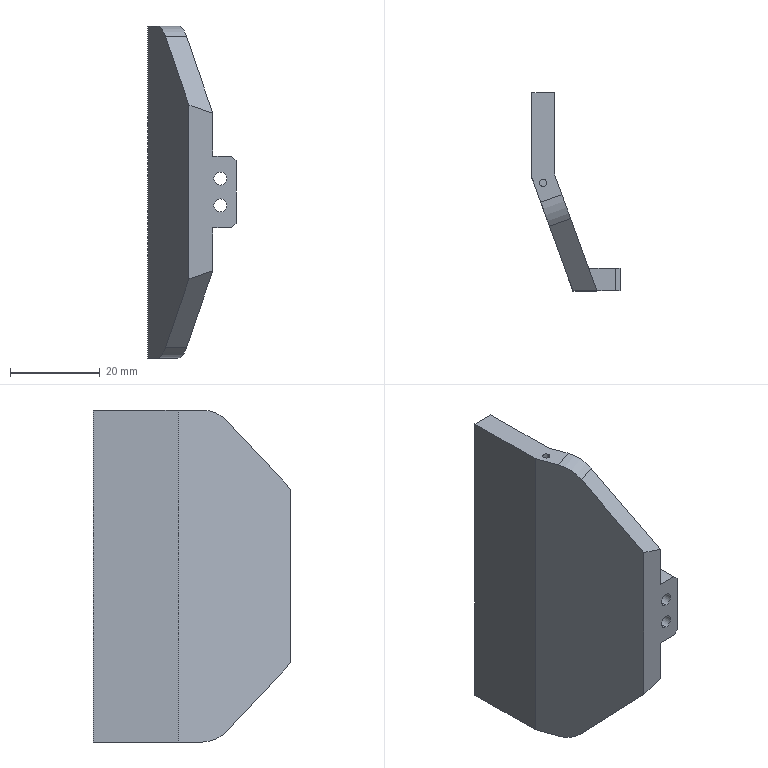NC program | NX | posted with a generic post | part box 19.643 x 44.061 x 74 mm
Lines 6014 to 6515 of 6515:
(FLOOR_FACING , TOOL : D8精光)
N12026 T03 M6
N12028 G54
N12030 G17 G0 G90 X-46. Y40.058 B0. C0. S5500 M3
N12032 G43 Z30. H3
N12034 Z-12.643
N12036 G94 G1 Z-14.643 F800.
N12038 X-41.
N12040 X41.
N12042 Y35.029
N12044 X-41.
N12046 Y30.
N12048 X41.
N12050 X43.
N12052 Z-12.643
N12054 G0 Z30.
(FLOOR_FACING_COPY , TOOL : D8精光)
N12056 X13. Y2.
N12058 Z2.
N12060 G1 Z0.
N12062 X11.
N12064 X-11.
N12066 X-13.
N12068 Z2.
N12070 G0 Z30.
(PLANAR_MILL_6_COPY , TOOL : D8精光)
N12072 X-12. Y9. S4500
N12074 Z-5.
N12076 G1 Z-7.
N12078 X-8.
N12080 X8.
N12082 X12.
N12084 Z-5.
N12086 G0 Z30.
N12088 X-12.
N12090 Z-5.
N12092 G1 Z-7.
N12094 X-8.
N12096 X8.
N12098 X12.
N12100 Z-5.
N12102 G0 Z30.
(PLANAR_MILL_6 , TOOL : D8精光)
N12104 X43. Y40.118
N12106 Z-19.
N12108 G1 Z-21.
N12110 G3 X41. Y38.118 R2.
N12112 G1 Y19.674
N12114 G2 X40.986 Y19.34 R4.
N12116 X37.617 Y11.668 R10.966
N12118 X37.396 Y11.444 R4.
N12120 G1 X22.116 Y-2.915
N12122 G2 X19.377 Y-4. R4.
N12124 G1 X-19.377
N12126 G2 X-22.116 Y-2.915 R4.
N12128 G1 X-37.396 Y11.444
N12130 G2 X-37.617 Y11.668 R4.
N12132 X-40.986 Y19.34 R11.02
N12134 X-41. Y19.674 R4.
N12136 G1 Y38.118
N12138 G3 X-43. Y40.118 R2.
N12140 G1 Z-19.
N12142 G0 Z30.
N12144 X43.
N12146 Z-19.
N12148 G1 Z-21.
N12150 G3 X41. Y38.118 R2.
N12152 G1 Y19.674
N12154 G2 X40.986 Y19.34 R4.
N12156 X37.617 Y11.668 R10.966
N12158 X37.396 Y11.444 R4.
N12160 G1 X22.116 Y-2.915
N12162 G2 X19.377 Y-4. R4.
N12164 G1 X-19.377
N12166 G2 X-22.116 Y-2.915 R4.
N12168 G1 X-37.396 Y11.444
N12170 G2 X-37.617 Y11.668 R4.
N12172 X-40.986 Y19.34 R11.02
N12174 X-41. Y19.674 R4.
N12176 G1 Y38.118
N12178 G3 X-43. Y40.118 R2.
N12180 G1 Z-19.
N12182 G0 Z30.
N12184 M5
(CURVE_DRIVE_1 , TOOL : R1)
N12186 T04 M6
N12188 G54
N12190 G17 G0 G90 X-7.728 Y6.011 B0. C0. S4500 M3
N12192 G43 Z30. H4
N12194 Z2.798
N12196 G94 G1 Z0.675 F1000.
N12198 Y5.999 Z0.532
N12200 Y5.967 Z0.393
N12202 Y5.916 Z0.26
N12204 Y5.846 Z0.136
N12206 Y5.759 Z0.022
N12208 Y5.657 Z-0.077
N12210 Y5.542 Z-0.162
N12212 Y5.416 Z-0.229
N12214 Y5.282 Z-0.277
N12216 Y5.142 Z-0.306
N12218 Y5. Z-0.315
N12220 Y4.958 Z-0.314
N12222 Y0.043
N12224 Y0. Z-0.315
N12226 X-7.749 Z-0.336
N12228 Y0.041 Z-0.335
N12230 Y4.958
N12232 Y5. Z-0.336
N12234 X-7.771 Z-0.357
N12236 Y4.958 Z-0.356
N12238 Y0.043
N12240 Y0. Z-0.357
N12242 X-7.792 Z-0.378
N12244 Y0.043
N12246 Y4.958
N12248 Y5.
N12250 X-7.813 Z-0.399
N12252 Y4.958
N12254 Y0.043
N12256 Y0.
N12258 X-7.834 Z-0.42
N12260 Y0.043
N12262 Y4.958
N12264 Y5.
N12266 X-7.855 Z-0.442
N12268 Y4.958 Z-0.441
N12270 Y0.043
N12272 Y0. Z-0.442
N12274 X-7.877 Z-0.463
N12276 Y0.043 Z-0.462
N12278 Y4.958
N12280 Y5. Z-0.463
N12282 X-7.898 Z-0.484
N12284 Y4.955
N12286 Y0.041
N12288 Y0.
N12290 X-7.919 Z-0.505
N12292 Y0.043
N12294 Y4.958
N12296 Y5.
N12298 X-7.94 Z-0.526
N12300 Y4.958
N12302 Y0.043
N12304 Y0.
N12306 X-7.961 Z-0.548
N12308 Y0.043 Z-0.547
N12310 Y4.958
N12312 Y5. Z-0.548
N12314 X-7.983 Z-0.569
N12316 Y4.958 Z-0.568
N12318 Y0.043
N12320 Y0. Z-0.569
N12322 X-8.004 Z-0.59
N12324 Y0.043
N12326 Y4.958
N12328 Y5.
N12330 X-8.025 Z-0.611
N12332 Y4.958
N12334 Y0.043
N12336 Y0.
N12338 X-8.046 Z-0.633
N12340 Y0.043 Z-0.632
N12342 Y4.958
N12344 Y5. Z-0.633
N12346 X-8.068 Z-0.654
N12348 Y4.958 Z-0.653
N12350 Y0.043
N12352 Y0. Z-0.654
N12354 X-8.089 Z-0.675
N12356 Y0.043
N12358 Y4.958
N12360 Y5.
N12362 X-8.11 Z-0.696
N12364 Y4.958
N12366 Y0.043
N12368 Y0.
N12370 X-8.131 Z-0.717
N12372 Y0.043
N12374 Y4.958
N12376 Y5.
N12378 X-8.152 Z-0.739
N12380 Y4.958 Z-0.738
N12382 Y0.043
N12384 Y0. Z-0.739
N12386 X-8.174 Z-0.76
N12388 Y0.043 Z-0.759
N12390 Y4.958
N12392 Y5. Z-0.76
N12394 X-8.195 Z-0.781
N12396 Y4.958
N12398 Y0.043
N12400 Y0.
N12402 X-8.216 Z-0.802
N12404 Y0.043
N12406 Y4.958
N12408 Y5.
N12410 X-8.237 Z-0.823
N12412 Y4.958
N12414 Y0.043
N12416 Y0.
N12418 X-8.258 Z-0.845
N12420 Y0.043 Z-0.844
N12422 Y4.958
N12424 Y5. Z-0.845
N12426 X-8.28 Z-0.866
N12428 Y4.958 Z-0.865
N12430 Y0.043
N12432 Y0. Z-0.866
N12434 X-8.301 Z-0.887
N12436 Y0.043
N12438 Y4.958
N12440 Y5.
N12442 X-8.322 Z-0.908
N12444 Y4.958
N12446 Y0.043
N12448 Y0.
N12450 X-8.343 Z-0.93
N12452 Y0.043 Z-0.929
N12454 Y4.958
N12456 Y5. Z-0.93
N12458 X-8.364 Z-0.951
N12460 Y4.958 Z-0.95
N12462 X-8.365 Y0.043
N12464 Y0. Z-0.951
N12466 X-8.386 Z-0.972
N12468 Y0.043 Z-0.971
N12470 Y4.958
N12472 Y5. Z-0.972
N12474 X-8.407 Z-0.993
N12476 Y4.958
N12478 Y0.043
N12480 Y0.
N12482 X-8.428 Z-1.014
N12484 Y0.043
N12486 Y4.958
N12488 Y5.
N12490 X-8.449 Z-1.036
N12492 Y4.958 Z-1.035
N12494 Y0.043
N12496 Y0. Z-1.036
N12498 X-8.471 Z-1.057
N12500 Y0.043 Z-1.056
N12502 Y4.958
N12504 Y5. Z-1.057
N12506 X-8.492 Z-1.078
N12508 Y4.958
N12510 Y0.043
N12512 Y0.
N12514 X-8.513 Z-1.099
N12516 Y0.042
N12518 Y4.957
N12520 Y5.
N12522 X-8.534 Z-1.12
N12524 Y4.958
N12526 Y0.022
N12528 Y0.
N12530 X-8.555 Z-1.142
N12532 Y4.978 Z-1.141
N12534 Y5. Z-1.142
N12536 X-8.577 Z-1.163
N12538 Y4.958 Z-1.162
N12540 Y0. Z-1.163
N12542 X-8.598 Z-1.184
N12544 Y4.992
N12546 Y5.
N12548 X-8.619 Z-1.205
N12550 Y0.
N12552 X-8.64 Z-1.226
N12554 Y5.
N12556 X-8.661 Z-1.247
N12558 Y0.
N12560 X-8.682 Z-1.269
N12562 Y5.
N12564 X-8.703 Z-1.29
N12566 Y0.
N12568 Y-0.142 Z-1.282
N12570 Y-0.282 Z-1.253
N12572 Y-0.416 Z-1.204
N12574 Y-0.542 Z-1.137
N12576 Y-0.657 Z-1.053
N12578 Y-0.759 Z-0.953
N12580 Y-0.846 Z-0.84
N12582 Y-0.915 Z-0.715
N12584 Y-0.967 Z-0.582
N12586 Y-0.998 Z-0.443
N12588 Y-1.01 Z-0.301
N12590 Z2.472
N12592 G0 Z30.
N12594 X7.728 Y-1.011
N12596 Z2.798
N12598 G1 Z0.675
N12600 Y-0.999 Z0.532
N12602 Y-0.967 Z0.393
N12604 Y-0.916 Z0.26
N12606 Y-0.846 Z0.136
N12608 Y-0.759 Z0.022
N12610 Y-0.657 Z-0.077
N12612 Y-0.542 Z-0.162
N12614 Y-0.416 Z-0.229
N12616 Y-0.282 Z-0.277
N12618 Y-0.142 Z-0.306
N12620 Y0. Z-0.315
N12622 Y0.043 Z-0.314
N12624 Y4.958
N12626 Y5. Z-0.315
N12628 X7.749 Z-0.336
N12630 Y4.958 Z-0.335
N12632 Y0.043
N12634 Y0. Z-0.336
N12636 X7.771 Z-0.357
N12638 Y0.043 Z-0.356
N12640 Y4.958
N12642 Y5. Z-0.357
N12644 X7.792 Z-0.378
N12646 Y4.958
N12648 Y0.043
N12650 Y0.
N12652 X7.813 Z-0.399
N12654 Y0.043
N12656 Y4.958
N12658 Y5.
N12660 X7.834 Z-0.42
N12662 Y4.958
N12664 Y0.043
N12666 Y0.
N12668 X7.855 Z-0.442
N12670 Y0.043 Z-0.441
N12672 Y4.958
N12674 Y5. Z-0.442
N12676 X7.877 Z-0.463
N12678 Y4.958 Z-0.462
N12680 Y0.043
N12682 Y0. Z-0.463
N12684 X7.898 Z-0.484
N12686 Y0.045
N12688 Y4.959
N12690 Y5.
N12692 X7.919 Z-0.505
N12694 Y4.958
N12696 Y0.043
N12698 Y0.
N12700 X7.94 Z-0.526
N12702 Y0.043
N12704 Y4.958
N12706 Y5.
N12708 X7.961 Z-0.548
N12710 Y4.958 Z-0.547
N12712 Y0.043
N12714 Y0. Z-0.548
N12716 X7.983 Z-0.569
N12718 Y0.043 Z-0.568
N12720 Y4.958
N12722 Y5. Z-0.569
N12724 X8.004 Z-0.59
N12726 Y4.958
N12728 Y0.043
N12730 Y0.
N12732 X8.025 Z-0.611
N12734 Y0.043
N12736 Y4.958
N12738 Y5.
N12740 X8.046 Z-0.633
N12742 Y4.96 Z-0.632
N12744 Y0.043
N12746 Y0. Z-0.633
N12748 X8.068 Z-0.654
N12750 Y0.043 Z-0.653
N12752 Y4.958
N12754 Y5. Z-0.654
N12756 X8.089 Z-0.675
N12758 Y4.958
N12760 Y0.043
N12762 Y0.
N12764 X8.11 Z-0.696
N12766 Y0.043
N12768 Y4.958
N12770 Y5.
N12772 X8.131 Z-0.717
N12774 Y4.958
N12776 Y0.043
N12778 Y0.
N12780 X8.152 Z-0.739
N12782 Y0.043 Z-0.738
N12784 Y4.958
N12786 Y5. Z-0.739
N12788 X8.174 Z-0.76
N12790 Y4.958 Z-0.759
N12792 Y0.043
N12794 Y0. Z-0.76
N12796 X8.195 Z-0.781
N12798 Y0.043
N12800 Y4.958
N12802 Y5.
N12804 X8.216 Z-0.802
N12806 Y4.958
N12808 Y0.043
N12810 Y0.
N12812 X8.237 Z-0.823
N12814 Y0.043
N12816 Y4.958
N12818 Y5.
N12820 X8.258 Z-0.845
N12822 Y4.958 Z-0.844
N12824 Y0.043
N12826 Y0. Z-0.845
N12828 X8.28 Z-0.866
N12830 Y0.043 Z-0.865
N12832 Y4.958
N12834 Y5. Z-0.866
N12836 X8.301 Z-0.887
N12838 Y4.958
N12840 Y0.043
N12842 Y0.
N12844 X8.322 Z-0.908
N12846 Y0.043
N12848 Y4.958
N12850 Y5.
N12852 X8.343 Z-0.93
N12854 Y4.958 Z-0.929
N12856 Y0.043
N12858 Y0. Z-0.93
N12860 X8.365 Z-0.951
N12862 Y0.043 Z-0.95
N12864 Y4.96
N12866 Y5. Z-0.951
N12868 X8.386 Z-0.972
N12870 Y4.958
N12872 Y0.043
N12874 Y0.
N12876 X8.407 Z-0.993
N12878 Y0.043
N12880 Y4.958
N12882 Y5.
N12884 X8.428 Z-1.014
N12886 Y4.958
N12888 Y0.043
N12890 Y0.
N12892 X8.449 Z-1.036
N12894 Y0.043 Z-1.035
N12896 Y4.958
N12898 Y5. Z-1.036
N12900 X8.471 Z-1.057
N12902 Y4.958 Z-1.056
N12904 Y0.043
N12906 Y0. Z-1.057
N12908 X8.492 Z-1.078
N12910 Y0.043
N12912 Y4.958
N12914 Y5.
N12916 X8.513 Z-1.099
N12918 Y4.958
N12920 Y0.043
N12922 Y0.
N12924 X8.534 Z-1.12
N12926 Y0.043
N12928 Y4.966
N12930 Y5.
N12932 X8.555 Z-1.142
N12934 Y0.043 Z-1.141
N12936 Y0. Z-1.142
N12938 X8.577 Z-1.163
N12940 Y0.043 Z-1.162
N12942 Y5. Z-1.163
N12944 X8.598 Z-1.184
N12946 Y0.008
N12948 Y0.
N12950 X8.619 Z-1.205
N12952 Y5.
N12954 X8.64 Z-1.226
N12956 Y0.
N12958 X8.661 Z-1.247
N12960 Y5.
N12962 X8.682 Z-1.269
N12964 Y0.
N12966 X8.703 Z-1.29
N12968 Y5.
N12970 Y5.142 Z-1.282
N12972 Y5.282 Z-1.253
N12974 Y5.416 Z-1.204
N12976 Y5.542 Z-1.137
N12978 Y5.657 Z-1.053
N12980 Y5.759 Z-0.953
N12982 Y5.846 Z-0.84
N12984 Y5.916 Z-0.715
N12986 Y5.967 Z-0.582
N12988 Y5.998 Z-0.443
N12990 Y6.01 Z-0.301
N12992 Z2.472
N12994 G0 Z30.
N12996 M5
N12998 M2